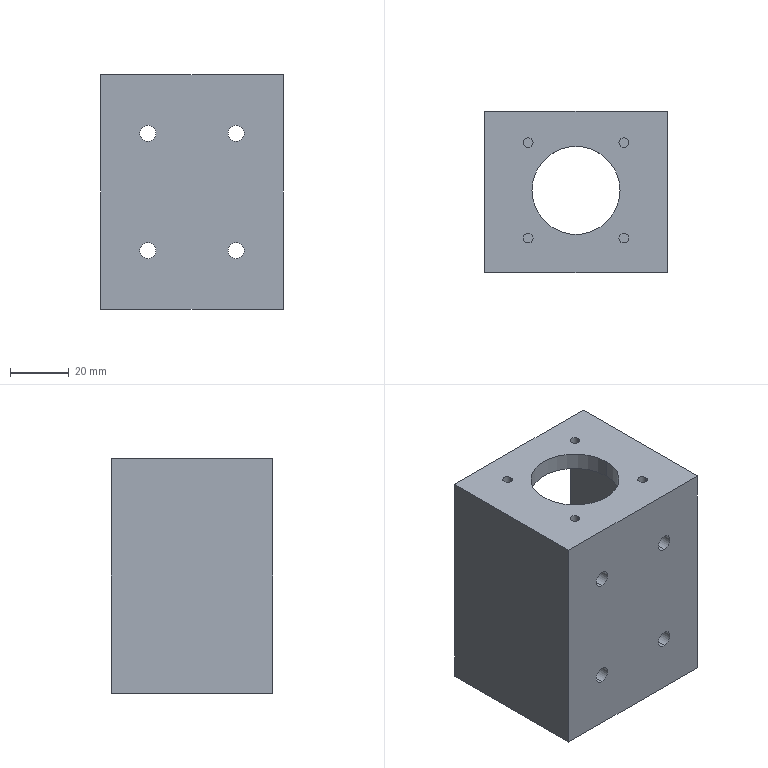Part | Creo | features CURVE 6, CUT 4, DATUM PLANE 3, PROTRUSION 2, CHAMFER 1, COORDINATE SYSTEM 1 | 1 solid | 45 faces | box 62 x 55 x 80 mm | volume 96326 mm3 | cylinder 26 | plane 19 | commonest cylinder face diameters 3.3 x8 5.5 x8 4.2 x6 30 x2 34 x2
STEP:
#1=CARTESIAN_POINT('',(0.,0.,0.));
#2=DIRECTION('',(0.,0.,1.));
#3=DIRECTION('',(1.,0.,0.));
#4=AXIS2_PLACEMENT_3D('',#1,#2,#3);
#5=CARTESIAN_POINT('',(31.,27.,0.));
#6=VERTEX_POINT('',#5);
#7=CARTESIAN_POINT('',(-31.,27.,0.));
#8=VERTEX_POINT('',#7);
#9=CARTESIAN_POINT('',(31.,27.,0.));
#10=DIRECTION('',(-1.,0.,0.));
#11=VECTOR('',#10,62.);
#12=LINE('',#9,#11);
#13=EDGE_CURVE('',#6,#8,#12,.T.);
#14=ORIENTED_EDGE('',*,*,#13,.T.);
#15=CARTESIAN_POINT('',(-31.,-28.,0.));
#16=VERTEX_POINT('',#15);
#17=CARTESIAN_POINT('',(-31.,27.,0.));
#18=DIRECTION('',(0.,-1.,0.));
#19=VECTOR('',#18,55.);
#20=LINE('',#17,#19);
#21=EDGE_CURVE('',#8,#16,#20,.T.);
#22=ORIENTED_EDGE('',*,*,#21,.T.);
#23=CARTESIAN_POINT('',(31.,-28.,0.));
#24=VERTEX_POINT('',#23);
#25=CARTESIAN_POINT('',(-31.,-28.,0.));
#26=DIRECTION('',(1.,0.,0.));
#27=VECTOR('',#26,62.);
#28=LINE('',#25,#27);
#29=EDGE_CURVE('',#16,#24,#28,.T.);
#30=ORIENTED_EDGE('',*,*,#29,.T.);
#31=CARTESIAN_POINT('',(31.,-28.,0.));
#32=DIRECTION('',(0.,1.,0.));
#33=VECTOR('',#32,55.);
#34=LINE('',#31,#33);
#35=EDGE_CURVE('',#24,#6,#34,.T.);
#36=ORIENTED_EDGE('',*,*,#35,.T.);
#37=EDGE_LOOP('',(#14,#22,#30,#36));
#38=FACE_OUTER_BOUND('',#37,.F.);
#39=CARTESIAN_POINT('',(0.,-17.,0.));
#40=VERTEX_POINT('',#39);
#41=CARTESIAN_POINT('',(0.,17.,0.));
#42=VERTEX_POINT('',#41);
#43=CARTESIAN_POINT('',(0.,0.,0.));
#44=DIRECTION('',(0.,0.,-1.));
#45=DIRECTION('',(0.,-1.,0.));
#46=AXIS2_PLACEMENT_3D('',#43,#44,#45);
#47=CIRCLE('',#46,17.);
#48=EDGE_CURVE('',#40,#42,#47,.T.);
#49=ORIENTED_EDGE('',*,*,#48,.T.);
#50=CARTESIAN_POINT('',(0.,0.,0.));
#51=DIRECTION('',(0.,0.,-1.));
#52=DIRECTION('',(0.,1.,0.));
#53=AXIS2_PLACEMENT_3D('',#50,#51,#52);
#54=CIRCLE('',#53,17.);
#55=EDGE_CURVE('',#42,#40,#54,.T.);
#56=ORIENTED_EDGE('',*,*,#55,.T.);
#57=EDGE_LOOP('',(#49,#56));
#58=FACE_BOUND('',#57,.F.);
#59=CARTESIAN_POINT('',(0.,18.9,0.));
#60=VERTEX_POINT('',#59);
#61=CARTESIAN_POINT('',(0.,23.1,0.));
#62=VERTEX_POINT('',#61);
#63=CARTESIAN_POINT('',(0.,21.,0.));
#64=DIRECTION('',(0.,0.,-1.));
#65=DIRECTION('',(0.,-1.,0.));
#66=AXIS2_PLACEMENT_3D('',#63,#64,#65);
#67=CIRCLE('',#66,2.1);
#68=EDGE_CURVE('',#60,#62,#67,.T.);
#69=ORIENTED_EDGE('',*,*,#68,.T.);
#70=CARTESIAN_POINT('',(0.,21.,0.));
#71=DIRECTION('',(0.,0.,-1.));
#72=DIRECTION('',(0.,1.,0.));
#73=AXIS2_PLACEMENT_3D('',#70,#71,#72);
#74=CIRCLE('',#73,2.1);
#75=EDGE_CURVE('',#62,#60,#74,.T.);
#76=ORIENTED_EDGE('',*,*,#75,.T.);
#77=EDGE_LOOP('',(#69,#76));
#78=FACE_BOUND('',#77,.F.);
#79=CARTESIAN_POINT('',(-18.187,-12.6,0.));
#80=VERTEX_POINT('',#79);
#81=CARTESIAN_POINT('',(-18.187,-8.4,0.));
#82=VERTEX_POINT('',#81);
#83=CARTESIAN_POINT('',(-18.187,-10.5,0.));
#84=DIRECTION('',(0.,0.,-1.));
#85=DIRECTION('',(0.,-1.,0.));
#86=AXIS2_PLACEMENT_3D('',#83,#84,#85);
#87=CIRCLE('',#86,2.1);
#88=EDGE_CURVE('',#80,#82,#87,.T.);
#89=ORIENTED_EDGE('',*,*,#88,.T.);
#90=CARTESIAN_POINT('',(-18.187,-10.5,0.));
#91=DIRECTION('',(0.,0.,-1.));
#92=DIRECTION('',(0.,1.,0.));
#93=AXIS2_PLACEMENT_3D('',#90,#91,#92);
#94=CIRCLE('',#93,2.1);
#95=EDGE_CURVE('',#82,#80,#94,.T.);
#96=ORIENTED_EDGE('',*,*,#95,.T.);
#97=EDGE_LOOP('',(#89,#96));
#98=FACE_BOUND('',#97,.F.);
#99=CARTESIAN_POINT('',(18.187,-12.6,0.));
#100=VERTEX_POINT('',#99);
#101=CARTESIAN_POINT('',(18.187,-8.4,0.));
#102=VERTEX_POINT('',#101);
#103=CARTESIAN_POINT('',(18.187,-10.5,0.));
#104=DIRECTION('',(0.,0.,-1.));
#105=DIRECTION('',(0.,-1.,0.));
#106=AXIS2_PLACEMENT_3D('',#103,#104,#105);
#107=CIRCLE('',#106,2.1);
#108=EDGE_CURVE('',#100,#102,#107,.T.);
#109=ORIENTED_EDGE('',*,*,#108,.T.);
#110=CARTESIAN_POINT('',(18.187,-10.5,0.));
#111=DIRECTION('',(0.,0.,-1.));
#112=DIRECTION('',(0.,1.,0.));
#113=AXIS2_PLACEMENT_3D('',#110,#111,#112);
#114=CIRCLE('',#113,2.1);
#115=EDGE_CURVE('',#102,#100,#114,.T.);
#116=ORIENTED_EDGE('',*,*,#115,.T.);
#117=EDGE_LOOP('',(#109,#116));
#118=FACE_BOUND('',#117,.F.);
#119=CARTESIAN_POINT('',(0.,0.,0.));
#120=DIRECTION('',(0.,0.,1.));
#121=DIRECTION('',(1.,0.,0.));
#122=AXIS2_PLACEMENT_3D('',#119,#120,#121);
#123=PLANE('',#122);
#124=ADVANCED_FACE('',(#38,#58,#78,#98,#118),#123,.F.);
#125=ORIENTED_EDGE('',*,*,#13,.F.);
#126=CARTESIAN_POINT('',(31.,27.,80.));
#127=VERTEX_POINT('',#126);
#128=CARTESIAN_POINT('',(31.,27.,0.));
#129=DIRECTION('',(0.,0.,1.));
#130=VECTOR('',#129,80.);
#131=LINE('',#128,#130);
#132=EDGE_CURVE('',#6,#127,#131,.T.);
#133=ORIENTED_EDGE('',*,*,#132,.T.);
#134=CARTESIAN_POINT('',(-31.,27.,80.));
#135=VERTEX_POINT('',#134);
#136=CARTESIAN_POINT('',(31.,27.,80.));
#137=DIRECTION('',(-1.,0.,0.));
#138=VECTOR('',#137,62.);
#139=LINE('',#136,#138);
#140=EDGE_CURVE('',#127,#135,#139,.T.);
#141=ORIENTED_EDGE('',*,*,#140,.T.);
#142=CARTESIAN_POINT('',(-31.,27.,0.));
#143=DIRECTION('',(0.,0.,1.));
#144=VECTOR('',#143,80.);
#145=LINE('',#142,#144);
#146=EDGE_CURVE('',#8,#135,#145,.T.);
#147=ORIENTED_EDGE('',*,*,#146,.F.);
#148=EDGE_LOOP('',(#125,#133,#141,#147));
#149=FACE_OUTER_BOUND('',#148,.F.);
#150=CARTESIAN_POINT('',(-25.,27.,8.));
#151=VERTEX_POINT('',#150);
#152=CARTESIAN_POINT('',(-25.,27.,72.));
#153=VERTEX_POINT('',#152);
#154=CARTESIAN_POINT('',(-25.,27.,8.));
#155=DIRECTION('',(0.,0.,1.));
#156=VECTOR('',#155,64.);
#157=LINE('',#154,#156);
#158=EDGE_CURVE('',#151,#153,#157,.T.);
#159=ORIENTED_EDGE('',*,*,#158,.T.);
#160=CARTESIAN_POINT('',(-23.,27.,74.));
#161=VERTEX_POINT('',#160);
#162=CARTESIAN_POINT('',(-23.,27.,74.));
#163=DIRECTION('',(-0.7071,0.,-0.7071));
#164=VECTOR('',#163,2.828);
#165=LINE('',#162,#164);
#166=EDGE_CURVE('',#161,#153,#165,.T.);
#167=ORIENTED_EDGE('',*,*,#166,.F.);
#168=CARTESIAN_POINT('',(23.,27.,74.));
#169=VERTEX_POINT('',#168);
#170=CARTESIAN_POINT('',(-23.,27.,74.));
#171=DIRECTION('',(1.,0.,0.));
#172=VECTOR('',#171,46.);
#173=LINE('',#170,#172);
#174=EDGE_CURVE('',#161,#169,#173,.T.);
#175=ORIENTED_EDGE('',*,*,#174,.T.);
#176=CARTESIAN_POINT('',(25.,27.,72.));
#177=VERTEX_POINT('',#176);
#178=CARTESIAN_POINT('',(25.,27.,72.));
#179=DIRECTION('',(-0.7071,0.,0.7071));
#180=VECTOR('',#179,2.828);
#181=LINE('',#178,#180);
#182=EDGE_CURVE('',#177,#169,#181,.T.);
#183=ORIENTED_EDGE('',*,*,#182,.F.);
#184=CARTESIAN_POINT('',(25.,27.,8.));
#185=VERTEX_POINT('',#184);
#186=CARTESIAN_POINT('',(25.,27.,72.));
#187=DIRECTION('',(0.,0.,-1.));
#188=VECTOR('',#187,64.);
#189=LINE('',#186,#188);
#190=EDGE_CURVE('',#177,#185,#189,.T.);
#191=ORIENTED_EDGE('',*,*,#190,.T.);
#192=CARTESIAN_POINT('',(23.,27.,6.));
#193=VERTEX_POINT('',#192);
#194=CARTESIAN_POINT('',(23.,27.,6.));
#195=DIRECTION('',(0.7071,0.,0.7071));
#196=VECTOR('',#195,2.828);
#197=LINE('',#194,#196);
#198=EDGE_CURVE('',#193,#185,#197,.T.);
#199=ORIENTED_EDGE('',*,*,#198,.F.);
#200=CARTESIAN_POINT('',(-23.,27.,6.));
#201=VERTEX_POINT('',#200);
#202=CARTESIAN_POINT('',(23.,27.,6.));
#203=DIRECTION('',(-1.,0.,0.));
#204=VECTOR('',#203,46.);
#205=LINE('',#202,#204);
#206=EDGE_CURVE('',#193,#201,#205,.T.);
#207=ORIENTED_EDGE('',*,*,#206,.T.);
#208=CARTESIAN_POINT('',(-25.,27.,8.));
#209=DIRECTION('',(0.7071,0.,-0.7071));
#210=VECTOR('',#209,2.828);
#211=LINE('',#208,#210);
#212=EDGE_CURVE('',#151,#201,#211,.T.);
#213=ORIENTED_EDGE('',*,*,#212,.F.);
#214=EDGE_LOOP('',(#159,#167,#175,#183,#191,#199,#207,#213));
#215=FACE_BOUND('',#214,.F.);
#216=CARTESIAN_POINT('',(31.,27.,0.));
#217=DIRECTION('',(0.,1.,0.));
#218=DIRECTION('',(-1.,0.,0.));
#219=AXIS2_PLACEMENT_3D('',#216,#217,#218);
#220=PLANE('',#219);
#221=ADVANCED_FACE('',(#149,#215),#220,.T.);
#222=ORIENTED_EDGE('',*,*,#35,.F.);
#223=CARTESIAN_POINT('',(31.,-28.,80.));
#224=VERTEX_POINT('',#223);
#225=CARTESIAN_POINT('',(31.,-28.,0.));
#226=DIRECTION('',(0.,0.,1.));
#227=VECTOR('',#226,80.);
#228=LINE('',#225,#227);
#229=EDGE_CURVE('',#24,#224,#228,.T.);
#230=ORIENTED_EDGE('',*,*,#229,.T.);
#231=CARTESIAN_POINT('',(31.,-28.,80.));
#232=DIRECTION('',(0.,1.,0.));
#233=VECTOR('',#232,55.);
#234=LINE('',#231,#233);
#235=EDGE_CURVE('',#224,#127,#234,.T.);
#236=ORIENTED_EDGE('',*,*,#235,.T.);
#237=ORIENTED_EDGE('',*,*,#132,.F.);
#238=EDGE_LOOP('',(#222,#230,#236,#237));
#239=FACE_OUTER_BOUND('',#238,.F.);
#240=CARTESIAN_POINT('',(31.,-28.,0.));
#241=DIRECTION('',(1.,0.,0.));
#242=DIRECTION('',(0.,1.,0.));
#243=AXIS2_PLACEMENT_3D('',#240,#241,#242);
#244=PLANE('',#243);
#245=ADVANCED_FACE('',(#239),#244,.T.);
#246=ORIENTED_EDGE('',*,*,#29,.F.);
#247=CARTESIAN_POINT('',(-31.,-28.,80.));
#248=VERTEX_POINT('',#247);
#249=CARTESIAN_POINT('',(-31.,-28.,0.));
#250=DIRECTION('',(0.,0.,1.));
#251=VECTOR('',#250,80.);
#252=LINE('',#249,#251);
#253=EDGE_CURVE('',#16,#248,#252,.T.);
#254=ORIENTED_EDGE('',*,*,#253,.T.);
#255=CARTESIAN_POINT('',(-31.,-28.,80.));
#256=DIRECTION('',(1.,0.,0.));
#257=VECTOR('',#256,62.);
#258=LINE('',#255,#257);
#259=EDGE_CURVE('',#248,#224,#258,.T.);
#260=ORIENTED_EDGE('',*,*,#259,.T.);
#261=ORIENTED_EDGE('',*,*,#229,.F.);
#262=EDGE_LOOP('',(#246,#254,#260,#261));
#263=FACE_OUTER_BOUND('',#262,.F.);
#264=CARTESIAN_POINT('',(-15.,-28.,57.25));
#265=VERTEX_POINT('',#264);
#266=CARTESIAN_POINT('',(-15.,-28.,62.75));
#267=VERTEX_POINT('',#266);
#268=CARTESIAN_POINT('',(-15.,-28.,60.));
#269=DIRECTION('',(0.,1.,0.));
#270=DIRECTION('',(0.,0.,-1.));
#271=AXIS2_PLACEMENT_3D('',#268,#269,#270);
#272=CIRCLE('',#271,2.75);
#273=EDGE_CURVE('',#265,#267,#272,.T.);
#274=ORIENTED_EDGE('',*,*,#273,.F.);
#275=CARTESIAN_POINT('',(-15.,-28.,60.));
#276=DIRECTION('',(0.,1.,0.));
#277=DIRECTION('',(0.,0.,1.));
#278=AXIS2_PLACEMENT_3D('',#275,#276,#277);
#279=CIRCLE('',#278,2.75);
#280=EDGE_CURVE('',#267,#265,#279,.T.);
#281=ORIENTED_EDGE('',*,*,#280,.F.);
#282=EDGE_LOOP('',(#274,#281));
#283=FACE_BOUND('',#282,.F.);
#284=CARTESIAN_POINT('',(-15.,-28.,17.25));
#285=VERTEX_POINT('',#284);
#286=CARTESIAN_POINT('',(-15.,-28.,22.75));
#287=VERTEX_POINT('',#286);
#288=CARTESIAN_POINT('',(-15.,-28.,20.));
#289=DIRECTION('',(0.,1.,0.));
#290=DIRECTION('',(0.,0.,-1.));
#291=AXIS2_PLACEMENT_3D('',#288,#289,#290);
#292=CIRCLE('',#291,2.75);
#293=EDGE_CURVE('',#285,#287,#292,.T.);
#294=ORIENTED_EDGE('',*,*,#293,.F.);
#295=CARTESIAN_POINT('',(-15.,-28.,20.));
#296=DIRECTION('',(0.,1.,0.));
#297=DIRECTION('',(0.,0.,1.));
#298=AXIS2_PLACEMENT_3D('',#295,#296,#297);
#299=CIRCLE('',#298,2.75);
#300=EDGE_CURVE('',#287,#285,#299,.T.);
#301=ORIENTED_EDGE('',*,*,#300,.F.);
#302=EDGE_LOOP('',(#294,#301));
#303=FACE_BOUND('',#302,.F.);
#304=CARTESIAN_POINT('',(15.,-28.,17.25));
#305=VERTEX_POINT('',#304);
#306=CARTESIAN_POINT('',(15.,-28.,22.75));
#307=VERTEX_POINT('',#306);
#308=CARTESIAN_POINT('',(15.,-28.,20.));
#309=DIRECTION('',(0.,1.,0.));
#310=DIRECTION('',(0.,0.,-1.));
#311=AXIS2_PLACEMENT_3D('',#308,#309,#310);
#312=CIRCLE('',#311,2.75);
#313=EDGE_CURVE('',#305,#307,#312,.T.);
#314=ORIENTED_EDGE('',*,*,#313,.F.);
#315=CARTESIAN_POINT('',(15.,-28.,20.));
#316=DIRECTION('',(0.,1.,0.));
#317=DIRECTION('',(0.,0.,1.));
#318=AXIS2_PLACEMENT_3D('',#315,#316,#317);
#319=CIRCLE('',#318,2.75);
#320=EDGE_CURVE('',#307,#305,#319,.T.);
#321=ORIENTED_EDGE('',*,*,#320,.F.);
#322=EDGE_LOOP('',(#314,#321));
#323=FACE_BOUND('',#322,.F.);
#324=CARTESIAN_POINT('',(15.,-28.,57.25));
#325=VERTEX_POINT('',#324);
#326=CARTESIAN_POINT('',(15.,-28.,62.75));
#327=VERTEX_POINT('',#326);
#328=CARTESIAN_POINT('',(15.,-28.,60.));
#329=DIRECTION('',(0.,1.,0.));
#330=DIRECTION('',(0.,0.,-1.));
#331=AXIS2_PLACEMENT_3D('',#328,#329,#330);
#332=CIRCLE('',#331,2.75);
#333=EDGE_CURVE('',#325,#327,#332,.T.);
#334=ORIENTED_EDGE('',*,*,#333,.F.);
#335=CARTESIAN_POINT('',(15.,-28.,60.));
#336=DIRECTION('',(0.,1.,0.));
#337=DIRECTION('',(0.,0.,1.));
#338=AXIS2_PLACEMENT_3D('',#335,#336,#337);
#339=CIRCLE('',#338,2.75);
#340=EDGE_CURVE('',#327,#325,#339,.T.);
#341=ORIENTED_EDGE('',*,*,#340,.F.);
#342=EDGE_LOOP('',(#334,#341));
#343=FACE_BOUND('',#342,.F.);
#344=CARTESIAN_POINT('',(-31.,-28.,0.));
#345=DIRECTION('',(0.,-1.,0.));
#346=DIRECTION('',(1.,0.,0.));
#347=AXIS2_PLACEMENT_3D('',#344,#345,#346);
#348=PLANE('',#347);
#349=ADVANCED_FACE('',(#263,#283,#303,#323,#343),#348,.T.);
#350=ORIENTED_EDGE('',*,*,#21,.F.);
#351=ORIENTED_EDGE('',*,*,#146,.T.);
#352=CARTESIAN_POINT('',(-31.,27.,80.));
#353=DIRECTION('',(0.,-1.,0.));
#354=VECTOR('',#353,55.);
#355=LINE('',#352,#354);
#356=EDGE_CURVE('',#135,#248,#355,.T.);
#357=ORIENTED_EDGE('',*,*,#356,.T.);
#358=ORIENTED_EDGE('',*,*,#253,.F.);
#359=EDGE_LOOP('',(#350,#351,#357,#358));
#360=FACE_OUTER_BOUND('',#359,.F.);
#361=CARTESIAN_POINT('',(-31.,27.,0.));
#362=DIRECTION('',(-1.,0.,0.));
#363=DIRECTION('',(0.,-1.,0.));
#364=AXIS2_PLACEMENT_3D('',#361,#362,#363);
#365=PLANE('',#364);
#366=ADVANCED_FACE('',(#360),#365,.T.);
#367=ORIENTED_EDGE('',*,*,#140,.F.);
#368=ORIENTED_EDGE('',*,*,#235,.F.);
#369=ORIENTED_EDGE('',*,*,#259,.F.);
#370=ORIENTED_EDGE('',*,*,#356,.F.);
#371=EDGE_LOOP('',(#367,#368,#369,#370));
#372=FACE_OUTER_BOUND('',#371,.F.);
#373=CARTESIAN_POINT('',(-14.61,16.26,80.));
#374=VERTEX_POINT('',#373);
#375=CARTESIAN_POINT('',(-17.91,16.26,80.));
#376=VERTEX_POINT('',#375);
#377=CARTESIAN_POINT('',(-16.26,16.26,80.));
#378=DIRECTION('',(0.,0.,-1.));
#379=DIRECTION('',(1.,0.,0.));
#380=AXIS2_PLACEMENT_3D('',#377,#378,#379);
#381=CIRCLE('',#380,1.65);
#382=EDGE_CURVE('',#374,#376,#381,.T.);
#383=ORIENTED_EDGE('',*,*,#382,.F.);
#384=CARTESIAN_POINT('',(-16.26,16.26,80.));
#385=DIRECTION('',(0.,0.,-1.));
#386=DIRECTION('',(-1.,0.,0.));
#387=AXIS2_PLACEMENT_3D('',#384,#385,#386);
#388=CIRCLE('',#387,1.65);
#389=EDGE_CURVE('',#376,#374,#388,.T.);
#390=ORIENTED_EDGE('',*,*,#389,.F.);
#391=EDGE_LOOP('',(#383,#390));
#392=FACE_BOUND('',#391,.F.);
#393=CARTESIAN_POINT('',(17.91,16.26,80.));
#394=VERTEX_POINT('',#393);
#395=CARTESIAN_POINT('',(14.61,16.26,80.));
#396=VERTEX_POINT('',#395);
#397=CARTESIAN_POINT('',(16.26,16.26,80.));
#398=DIRECTION('',(0.,0.,-1.));
#399=DIRECTION('',(1.,0.,0.));
#400=AXIS2_PLACEMENT_3D('',#397,#398,#399);
#401=CIRCLE('',#400,1.65);
#402=EDGE_CURVE('',#394,#396,#401,.T.);
#403=ORIENTED_EDGE('',*,*,#402,.F.);
#404=CARTESIAN_POINT('',(16.26,16.26,80.));
#405=DIRECTION('',(0.,0.,-1.));
#406=DIRECTION('',(-1.,0.,0.));
#407=AXIS2_PLACEMENT_3D('',#404,#405,#406);
#408=CIRCLE('',#407,1.65);
#409=EDGE_CURVE('',#396,#394,#408,.T.);
#410=ORIENTED_EDGE('',*,*,#409,.F.);
#411=EDGE_LOOP('',(#403,#410));
#412=FACE_BOUND('',#411,.F.);
#413=CARTESIAN_POINT('',(17.91,-16.26,80.));
#414=VERTEX_POINT('',#413);
#415=CARTESIAN_POINT('',(14.61,-16.26,80.));
#416=VERTEX_POINT('',#415);
#417=CARTESIAN_POINT('',(16.26,-16.26,80.));
#418=DIRECTION('',(0.,0.,-1.));
#419=DIRECTION('',(1.,0.,0.));
#420=AXIS2_PLACEMENT_3D('',#417,#418,#419);
#421=CIRCLE('',#420,1.65);
#422=EDGE_CURVE('',#414,#416,#421,.T.);
#423=ORIENTED_EDGE('',*,*,#422,.F.);
#424=CARTESIAN_POINT('',(16.26,-16.26,80.));
#425=DIRECTION('',(0.,0.,-1.));
#426=DIRECTION('',(-1.,0.,0.));
#427=AXIS2_PLACEMENT_3D('',#424,#425,#426);
#428=CIRCLE('',#427,1.65);
#429=EDGE_CURVE('',#416,#414,#428,.T.);
#430=ORIENTED_EDGE('',*,*,#429,.F.);
#431=EDGE_LOOP('',(#423,#430));
#432=FACE_BOUND('',#431,.F.);
#433=CARTESIAN_POINT('',(-14.61,-16.26,80.));
#434=VERTEX_POINT('',#433);
#435=CARTESIAN_POINT('',(-17.91,-16.26,80.));
#436=VERTEX_POINT('',#435);
#437=CARTESIAN_POINT('',(-16.26,-16.26,80.));
#438=DIRECTION('',(0.,0.,-1.));
#439=DIRECTION('',(1.,0.,0.));
#440=AXIS2_PLACEMENT_3D('',#437,#438,#439);
#441=CIRCLE('',#440,1.65);
#442=EDGE_CURVE('',#434,#436,#441,.T.);
#443=ORIENTED_EDGE('',*,*,#442,.F.);
#444=CARTESIAN_POINT('',(-16.26,-16.26,80.));
#445=DIRECTION('',(0.,0.,-1.));
#446=DIRECTION('',(-1.,0.,0.));
#447=AXIS2_PLACEMENT_3D('',#444,#445,#446);
#448=CIRCLE('',#447,1.65);
#449=EDGE_CURVE('',#436,#434,#448,.T.);
#450=ORIENTED_EDGE('',*,*,#449,.F.);
#451=EDGE_LOOP('',(#443,#450));
#452=FACE_BOUND('',#451,.F.);
#453=CARTESIAN_POINT('',(15.,0.,80.));
#454=VERTEX_POINT('',#453);
#455=CARTESIAN_POINT('',(-15.,0.,80.));
#456=VERTEX_POINT('',#455);
#457=CARTESIAN_POINT('',(0.,0.,80.));
#458=DIRECTION('',(0.,0.,-1.));
#459=DIRECTION('',(1.,0.,0.));
#460=AXIS2_PLACEMENT_3D('',#457,#458,#459);
#461=CIRCLE('',#460,15.);
#462=EDGE_CURVE('',#454,#456,#461,.T.);
#463=ORIENTED_EDGE('',*,*,#462,.F.);
#464=CARTESIAN_POINT('',(0.,0.,80.));
#465=DIRECTION('',(0.,0.,-1.));
#466=DIRECTION('',(-1.,0.,0.));
#467=AXIS2_PLACEMENT_3D('',#464,#465,#466);
#468=CIRCLE('',#467,15.);
#469=EDGE_CURVE('',#456,#454,#468,.T.);
#470=ORIENTED_EDGE('',*,*,#469,.F.);
#471=EDGE_LOOP('',(#463,#470));
#472=FACE_BOUND('',#471,.F.);
#473=CARTESIAN_POINT('',(0.,0.,80.));
#474=DIRECTION('',(0.,0.,1.));
#475=DIRECTION('',(1.,0.,0.));
#476=AXIS2_PLACEMENT_3D('',#473,#474,#475);
#477=PLANE('',#476);
#478=ADVANCED_FACE('',(#372,#392,#412,#432,#452,#472),#477,.T.);
#479=CARTESIAN_POINT('',(-15.,0.,74.));
#480=VERTEX_POINT('',#479);
#481=CARTESIAN_POINT('',(15.,0.,74.));
#482=VERTEX_POINT('',#481);
#483=CARTESIAN_POINT('',(0.,0.,74.));
#484=DIRECTION('',(0.,0.,1.));
#485=DIRECTION('',(-1.,0.,0.));
#486=AXIS2_PLACEMENT_3D('',#483,#484,#485);
#487=CIRCLE('',#486,15.);
#488=EDGE_CURVE('',#480,#482,#487,.T.);
#489=ORIENTED_EDGE('',*,*,#488,.T.);
#490=CARTESIAN_POINT('',(15.,0.,74.));
#491=DIRECTION('',(0.,0.,1.));
#492=VECTOR('',#491,6.);
#493=LINE('',#490,#492);
#494=EDGE_CURVE('',#482,#454,#493,.T.);
#495=ORIENTED_EDGE('',*,*,#494,.T.);
#496=ORIENTED_EDGE('',*,*,#462,.T.);
#497=CARTESIAN_POINT('',(-15.,0.,74.));
#498=DIRECTION('',(0.,0.,1.));
#499=VECTOR('',#498,6.);
#500=LINE('',#497,#499);
#501=EDGE_CURVE('',#480,#456,#500,.T.);
#502=ORIENTED_EDGE('',*,*,#501,.F.);
#503=EDGE_LOOP('',(#489,#495,#496,#502));
#504=FACE_OUTER_BOUND('',#503,.F.);
#505=CARTESIAN_POINT('',(0.,0.,0.));
#506=DIRECTION('',(0.,0.,1.));
#507=DIRECTION('',(1.,0.,0.));
#508=AXIS2_PLACEMENT_3D('',#505,#506,#507);
#509=CYLINDRICAL_SURFACE('',#508,15.);
#510=ADVANCED_FACE('',(#504),#509,.F.);
#511=CARTESIAN_POINT('',(23.,-20.,74.));
#512=VERTEX_POINT('',#511);
#513=CARTESIAN_POINT('',(23.,27.,74.));
#514=DIRECTION('',(0.,-1.,0.));
#515=VECTOR('',#514,47.);
#516=LINE('',#513,#515);
#517=EDGE_CURVE('',#169,#512,#516,.T.);
#518=ORIENTED_EDGE('',*,*,#517,.F.);
#519=ORIENTED_EDGE('',*,*,#174,.F.);
#520=CARTESIAN_POINT('',(-23.,-20.,74.));
#521=VERTEX_POINT('',#520);
#522=CARTESIAN_POINT('',(-23.,27.,74.));
#523=DIRECTION('',(0.,-1.,0.));
#524=VECTOR('',#523,47.);
#525=LINE('',#522,#524);
#526=EDGE_CURVE('',#161,#521,#525,.T.);
#527=ORIENTED_EDGE('',*,*,#526,.T.);
#528=CARTESIAN_POINT('',(23.,-20.,74.));
#529=DIRECTION('',(-1.,0.,0.));
#530=VECTOR('',#529,46.);
#531=LINE('',#528,#530);
#532=EDGE_CURVE('',#512,#521,#531,.T.);
#533=ORIENTED_EDGE('',*,*,#532,.F.);
#534=EDGE_LOOP('',(#518,#519,#527,#533));
#535=FACE_OUTER_BOUND('',#534,.F.);
#536=CARTESIAN_POINT('',(-17.91,16.26,74.));
#537=VERTEX_POINT('',#536);
#538=CARTESIAN_POINT('',(-14.61,16.26,74.));
#539=VERTEX_POINT('',#538);
#540=CARTESIAN_POINT('',(-16.26,16.26,74.));
#541=DIRECTION('',(0.,0.,1.));
#542=DIRECTION('',(-1.,0.,0.));
#543=AXIS2_PLACEMENT_3D('',#540,#541,#542);
#544=CIRCLE('',#543,1.65);
#545=EDGE_CURVE('',#537,#539,#544,.T.);
#546=ORIENTED_EDGE('',*,*,#545,.F.);
#547=CARTESIAN_POINT('',(-16.26,16.26,74.));
#548=DIRECTION('',(0.,0.,1.));
#549=DIRECTION('',(1.,0.,0.));
#550=AXIS2_PLACEMENT_3D('',#547,#548,#549);
#551=CIRCLE('',#550,1.65);
#552=EDGE_CURVE('',#539,#537,#551,.T.);
#553=ORIENTED_EDGE('',*,*,#552,.F.);
#554=EDGE_LOOP('',(#546,#553));
#555=FACE_BOUND('',#554,.F.);
#556=CARTESIAN_POINT('',(14.61,16.26,74.));
#557=VERTEX_POINT('',#556);
#558=CARTESIAN_POINT('',(17.91,16.26,74.));
#559=VERTEX_POINT('',#558);
#560=CARTESIAN_POINT('',(16.26,16.26,74.));
#561=DIRECTION('',(0.,0.,1.));
#562=DIRECTION('',(-1.,0.,0.));
#563=AXIS2_PLACEMENT_3D('',#560,#561,#562);
#564=CIRCLE('',#563,1.65);
#565=EDGE_CURVE('',#557,#559,#564,.T.);
#566=ORIENTED_EDGE('',*,*,#565,.F.);
#567=CARTESIAN_POINT('',(16.26,16.26,74.));
#568=DIRECTION('',(0.,0.,1.));
#569=DIRECTION('',(1.,0.,0.));
#570=AXIS2_PLACEMENT_3D('',#567,#568,#569);
#571=CIRCLE('',#570,1.65);
#572=EDGE_CURVE('',#559,#557,#571,.T.);
#573=ORIENTED_EDGE('',*,*,#572,.F.);
#574=EDGE_LOOP('',(#566,#573));
#575=FACE_BOUND('',#574,.F.);
#576=CARTESIAN_POINT('',(14.61,-16.26,74.));
#577=VERTEX_POINT('',#576);
#578=CARTESIAN_POINT('',(17.91,-16.26,74.));
#579=VERTEX_POINT('',#578);
#580=CARTESIAN_POINT('',(16.26,-16.26,74.));
#581=DIRECTION('',(0.,0.,1.));
#582=DIRECTION('',(-1.,0.,0.));
#583=AXIS2_PLACEMENT_3D('',#580,#581,#582);
#584=CIRCLE('',#583,1.65);
#585=EDGE_CURVE('',#577,#579,#584,.T.);
#586=ORIENTED_EDGE('',*,*,#585,.F.);
#587=CARTESIAN_POINT('',(16.26,-16.26,74.));
#588=DIRECTION('',(0.,0.,1.));
#589=DIRECTION('',(1.,0.,0.));
#590=AXIS2_PLACEMENT_3D('',#587,#588,#589);
#591=CIRCLE('',#590,1.65);
#592=EDGE_CURVE('',#579,#577,#591,.T.);
#593=ORIENTED_EDGE('',*,*,#592,.F.);
#594=EDGE_LOOP('',(#586,#593));
#595=FACE_BOUND('',#594,.F.);
#596=CARTESIAN_POINT('',(-17.91,-16.26,74.));
#597=VERTEX_POINT('',#596);
#598=CARTESIAN_POINT('',(-14.61,-16.26,74.));
#599=VERTEX_POINT('',#598);
#600=CARTESIAN_POINT('',(-16.26,-16.26,74.));
#601=DIRECTION('',(0.,0.,1.));
#602=DIRECTION('',(-1.,0.,0.));
#603=AXIS2_PLACEMENT_3D('',#600,#601,#602);
#604=CIRCLE('',#603,1.65);
#605=EDGE_CURVE('',#597,#599,#604,.T.);
#606=ORIENTED_EDGE('',*,*,#605,.F.);
#607=CARTESIAN_POINT('',(-16.26,-16.26,74.));
#608=DIRECTION('',(0.,0.,1.));
#609=DIRECTION('',(1.,0.,0.));
#610=AXIS2_PLACEMENT_3D('',#607,#608,#609);
#611=CIRCLE('',#610,1.65);
#612=EDGE_CURVE('',#599,#597,#611,.T.);
#613=ORIENTED_EDGE('',*,*,#612,.F.);
#614=EDGE_LOOP('',(#606,#613));
#615=FACE_BOUND('',#614,.F.);
#616=ORIENTED_EDGE('',*,*,#488,.F.);
#617=CARTESIAN_POINT('',(0.,0.,74.));
#618=DIRECTION('',(0.,0.,1.));
#619=DIRECTION('',(1.,0.,0.));
#620=AXIS2_PLACEMENT_3D('',#617,#618,#619);
#621=CIRCLE('',#620,15.);
#622=EDGE_CURVE('',#482,#480,#621,.T.);
#623=ORIENTED_EDGE('',*,*,#622,.F.);
#624=EDGE_LOOP('',(#616,#623));
#625=FACE_BOUND('',#624,.F.);
#626=CARTESIAN_POINT('',(-25.,27.,74.));
#627=DIRECTION('',(0.,0.,1.));
#628=DIRECTION('',(1.,0.,0.));
#629=AXIS2_PLACEMENT_3D('',#626,#627,#628);
#630=PLANE('',#629);
#631=ADVANCED_FACE('',(#535,#555,#575,#595,#615,#625),#630,.F.);
#632=ORIENTED_EDGE('',*,*,#622,.T.);
#633=ORIENTED_EDGE('',*,*,#501,.T.);
#634=ORIENTED_EDGE('',*,*,#469,.T.);
#635=ORIENTED_EDGE('',*,*,#494,.F.);
#636=EDGE_LOOP('',(#632,#633,#634,#635));
#637=FACE_OUTER_BOUND('',#636,.F.);
#638=CARTESIAN_POINT('',(0.,0.,0.));
#639=DIRECTION('',(0.,0.,1.));
#640=DIRECTION('',(1.,0.,0.));
#641=AXIS2_PLACEMENT_3D('',#638,#639,#640);
#642=CYLINDRICAL_SURFACE('',#641,15.);
#643=ADVANCED_FACE('',(#637),#642,.F.);
#644=ORIENTED_EDGE('',*,*,#545,.T.);
#645=CARTESIAN_POINT('',(-14.61,16.26,74.));
#646=DIRECTION('',(0.,0.,1.));
#647=VECTOR('',#646,6.);
#648=LINE('',#645,#647);
#649=EDGE_CURVE('',#539,#374,#648,.T.);
#650=ORIENTED_EDGE('',*,*,#649,.T.);
#651=ORIENTED_EDGE('',*,*,#382,.T.);
#652=CARTESIAN_POINT('',(-17.91,16.26,74.));
#653=DIRECTION('',(0.,0.,1.));
#654=VECTOR('',#653,6.);
#655=LINE('',#652,#654);
#656=EDGE_CURVE('',#537,#376,#655,.T.);
#657=ORIENTED_EDGE('',*,*,#656,.F.);
#658=EDGE_LOOP('',(#644,#650,#651,#657));
#659=FACE_OUTER_BOUND('',#658,.F.);
#660=CARTESIAN_POINT('',(-16.26,16.26,0.));
#661=DIRECTION('',(0.,0.,1.));
#662=DIRECTION('',(1.,0.,0.));
#663=AXIS2_PLACEMENT_3D('',#660,#661,#662);
#664=CYLINDRICAL_SURFACE('',#663,1.65);
#665=ADVANCED_FACE('',(#659),#664,.F.);
#666=ORIENTED_EDGE('',*,*,#552,.T.);
#667=ORIENTED_EDGE('',*,*,#656,.T.);
#668=ORIENTED_EDGE('',*,*,#389,.T.);
#669=ORIENTED_EDGE('',*,*,#649,.F.);
#670=EDGE_LOOP('',(#666,#667,#668,#669));
#671=FACE_OUTER_BOUND('',#670,.F.);
#672=CARTESIAN_POINT('',(-16.26,16.26,0.));
#673=DIRECTION('',(0.,0.,1.));
#674=DIRECTION('',(1.,0.,0.));
#675=AXIS2_PLACEMENT_3D('',#672,#673,#674);
#676=CYLINDRICAL_SURFACE('',#675,1.65);
#677=ADVANCED_FACE('',(#671),#676,.F.);
#678=ORIENTED_EDGE('',*,*,#565,.T.);
#679=CARTESIAN_POINT('',(17.91,16.26,74.));
#680=DIRECTION('',(0.,0.,1.));
#681=VECTOR('',#680,6.);
#682=LINE('',#679,#681);
#683=EDGE_CURVE('',#559,#394,#682,.T.);
#684=ORIENTED_EDGE('',*,*,#683,.T.);
#685=ORIENTED_EDGE('',*,*,#402,.T.);
#686=CARTESIAN_POINT('',(14.61,16.26,74.));
#687=DIRECTION('',(0.,0.,1.));
#688=VECTOR('',#687,6.);
#689=LINE('',#686,#688);
#690=EDGE_CURVE('',#557,#396,#689,.T.);
#691=ORIENTED_EDGE('',*,*,#690,.F.);
#692=EDGE_LOOP('',(#678,#684,#685,#691));
#693=FACE_OUTER_BOUND('',#692,.F.);
#694=CARTESIAN_POINT('',(16.26,16.26,0.));
#695=DIRECTION('',(0.,0.,1.));
#696=DIRECTION('',(1.,0.,0.));
#697=AXIS2_PLACEMENT_3D('',#694,#695,#696);
#698=CYLINDRICAL_SURFACE('',#697,1.65);
#699=ADVANCED_FACE('',(#693),#698,.F.);
#700=ORIENTED_EDGE('',*,*,#572,.T.);
#701=ORIENTED_EDGE('',*,*,#690,.T.);
#702=ORIENTED_EDGE('',*,*,#409,.T.);
#703=ORIENTED_EDGE('',*,*,#683,.F.);
#704=EDGE_LOOP('',(#700,#701,#702,#703));
#705=FACE_OUTER_BOUND('',#704,.F.);
#706=CARTESIAN_POINT('',(16.26,16.26,0.));
#707=DIRECTION('',(0.,0.,1.));
#708=DIRECTION('',(1.,0.,0.));
#709=AXIS2_PLACEMENT_3D('',#706,#707,#708);
#710=CYLINDRICAL_SURFACE('',#709,1.65);
#711=ADVANCED_FACE('',(#705),#710,.F.);
#712=ORIENTED_EDGE('',*,*,#585,.T.);
#713=CARTESIAN_POINT('',(17.91,-16.26,74.));
#714=DIRECTION('',(0.,0.,1.));
#715=VECTOR('',#714,6.);
#716=LINE('',#713,#715);
#717=EDGE_CURVE('',#579,#414,#716,.T.);
#718=ORIENTED_EDGE('',*,*,#717,.T.);
#719=ORIENTED_EDGE('',*,*,#422,.T.);
#720=CARTESIAN_POINT('',(14.61,-16.26,74.));
#721=DIRECTION('',(0.,0.,1.));
#722=VECTOR('',#721,6.);
#723=LINE('',#720,#722);
#724=EDGE_CURVE('',#577,#416,#723,.T.);
#725=ORIENTED_EDGE('',*,*,#724,.F.);
#726=EDGE_LOOP('',(#712,#718,#719,#725));
#727=FACE_OUTER_BOUND('',#726,.F.);
#728=CARTESIAN_POINT('',(16.26,-16.26,0.));
#729=DIRECTION('',(0.,0.,1.));
#730=DIRECTION('',(1.,0.,0.));
#731=AXIS2_PLACEMENT_3D('',#728,#729,#730);
#732=CYLINDRICAL_SURFACE('',#731,1.65);
#733=ADVANCED_FACE('',(#727),#732,.F.);
#734=ORIENTED_EDGE('',*,*,#592,.T.);
#735=ORIENTED_EDGE('',*,*,#724,.T.);
#736=ORIENTED_EDGE('',*,*,#429,.T.);
#737=ORIENTED_EDGE('',*,*,#717,.F.);
#738=EDGE_LOOP('',(#734,#735,#736,#737));
#739=FACE_OUTER_BOUND('',#738,.F.);
#740=CARTESIAN_POINT('',(16.26,-16.26,0.));
#741=DIRECTION('',(0.,0.,1.));
#742=DIRECTION('',(1.,0.,0.));
#743=AXIS2_PLACEMENT_3D('',#740,#741,#742);
#744=CYLINDRICAL_SURFACE('',#743,1.65);
#745=ADVANCED_FACE('',(#739),#744,.F.);
#746=ORIENTED_EDGE('',*,*,#605,.T.);
#747=CARTESIAN_POINT('',(-14.61,-16.26,74.));
#748=DIRECTION('',(0.,0.,1.));
#749=VECTOR('',#748,6.);
#750=LINE('',#747,#749);
#751=EDGE_CURVE('',#599,#434,#750,.T.);
#752=ORIENTED_EDGE('',*,*,#751,.T.);
#753=ORIENTED_EDGE('',*,*,#442,.T.);
#754=CARTESIAN_POINT('',(-17.91,-16.26,74.));
#755=DIRECTION('',(0.,0.,1.));
#756=VECTOR('',#755,6.);
#757=LINE('',#754,#756);
#758=EDGE_CURVE('',#597,#436,#757,.T.);
#759=ORIENTED_EDGE('',*,*,#758,.F.);
#760=EDGE_LOOP('',(#746,#752,#753,#759));
#761=FACE_OUTER_BOUND('',#760,.F.);
#762=CARTESIAN_POINT('',(-16.26,-16.26,0.));
#763=DIRECTION('',(0.,0.,1.));
#764=DIRECTION('',(1.,0.,0.));
#765=AXIS2_PLACEMENT_3D('',#762,#763,#764);
#766=CYLINDRICAL_SURFACE('',#765,1.65);
#767=ADVANCED_FACE('',(#761),#766,.F.);
#768=ORIENTED_EDGE('',*,*,#612,.T.);
#769=ORIENTED_EDGE('',*,*,#758,.T.);
#770=ORIENTED_EDGE('',*,*,#449,.T.);
#771=ORIENTED_EDGE('',*,*,#751,.F.);
#772=EDGE_LOOP('',(#768,#769,#770,#771));
#773=FACE_OUTER_BOUND('',#772,.F.);
#774=CARTESIAN_POINT('',(-16.26,-16.26,0.));
#775=DIRECTION('',(0.,0.,1.));
#776=DIRECTION('',(1.,0.,0.));
#777=AXIS2_PLACEMENT_3D('',#774,#775,#776);
#778=CYLINDRICAL_SURFACE('',#777,1.65);
#779=ADVANCED_FACE('',(#773),#778,.F.);
#780=ORIENTED_EDGE('',*,*,#517,.T.);
#781=CARTESIAN_POINT('',(24.,-21.,73.));
#782=VERTEX_POINT('',#781);
#783=CARTESIAN_POINT('',(24.,-21.,73.));
#784=DIRECTION('',(-0.5774,0.5774,0.5774));
#785=VECTOR('',#784,1.732);
#786=LINE('',#783,#785);
#787=EDGE_CURVE('',#782,#512,#786,.T.);
#788=ORIENTED_EDGE('',*,*,#787,.F.);
#789=CARTESIAN_POINT('',(25.,-20.,72.));
#790=VERTEX_POINT('',#789);
#791=CARTESIAN_POINT('',(25.,-20.,72.));
#792=DIRECTION('',(-0.5774,-0.5774,0.5774));
#793=VECTOR('',#792,1.732);
#794=LINE('',#791,#793);
#795=EDGE_CURVE('',#790,#782,#794,.T.);
#796=ORIENTED_EDGE('',*,*,#795,.F.);
#797=CARTESIAN_POINT('',(25.,27.,72.));
#798=DIRECTION('',(0.,-1.,0.));
#799=VECTOR('',#798,47.);
#800=LINE('',#797,#799);
#801=EDGE_CURVE('',#177,#790,#800,.T.);
#802=ORIENTED_EDGE('',*,*,#801,.F.);
#803=ORIENTED_EDGE('',*,*,#182,.T.);
#804=EDGE_LOOP('',(#780,#788,#796,#802,#803));
#805=FACE_OUTER_BOUND('',#804,.F.);
#806=CARTESIAN_POINT('',(24.,2.5,73.));
#807=DIRECTION('',(-0.7071,0.,-0.7071));
#808=DIRECTION('',(0.7071,0.,-0.7071));
#809=AXIS2_PLACEMENT_3D('',#806,#807,#808);
#810=PLANE('',#809);
#811=ADVANCED_FACE('',(#805),#810,.T.);
#812=ORIENTED_EDGE('',*,*,#532,.T.);
#813=CARTESIAN_POINT('',(-24.,-21.,73.));
#814=VERTEX_POINT('',#813);
#815=CARTESIAN_POINT('',(-23.,-20.,74.));
#816=DIRECTION('',(-0.5774,-0.5774,-0.5774));
#817=VECTOR('',#816,1.732);
#818=LINE('',#815,#817);
#819=EDGE_CURVE('',#521,#814,#818,.T.);
#820=ORIENTED_EDGE('',*,*,#819,.T.);
#821=CARTESIAN_POINT('',(-23.,-22.,72.));
#822=VERTEX_POINT('',#821);
#823=CARTESIAN_POINT('',(-23.,-22.,72.));
#824=DIRECTION('',(-0.5774,0.5774,0.5774));
#825=VECTOR('',#824,1.732);
#826=LINE('',#823,#825);
#827=EDGE_CURVE('',#822,#814,#826,.T.);
#828=ORIENTED_EDGE('',*,*,#827,.F.);
#829=CARTESIAN_POINT('',(23.,-22.,72.));
#830=VERTEX_POINT('',#829);
#831=CARTESIAN_POINT('',(23.,-22.,72.));
#832=DIRECTION('',(-1.,0.,0.));
#833=VECTOR('',#832,46.);
#834=LINE('',#831,#833);
#835=EDGE_CURVE('',#830,#822,#834,.T.);
#836=ORIENTED_EDGE('',*,*,#835,.F.);
#837=CARTESIAN_POINT('',(23.,-22.,72.));
#838=DIRECTION('',(0.5774,0.5774,0.5774));
#839=VECTOR('',#838,1.732);
#840=LINE('',#837,#839);
#841=EDGE_CURVE('',#830,#782,#840,.T.);
#842=ORIENTED_EDGE('',*,*,#841,.T.);
#843=ORIENTED_EDGE('',*,*,#787,.T.);
#844=EDGE_LOOP('',(#812,#820,#828,#836,#842,#843));
#845=FACE_OUTER_BOUND('',#844,.F.);
#846=CARTESIAN_POINT('',(0.,-21.,73.));
#847=DIRECTION('',(0.,0.7071,-0.7071));
#848=DIRECTION('',(0.,-0.7071,-0.7071));
#849=AXIS2_PLACEMENT_3D('',#846,#847,#848);
#850=PLANE('',#849);
#851=ADVANCED_FACE('',(#845),#850,.T.);
#852=CARTESIAN_POINT('',(-25.,-20.,72.));
#853=VERTEX_POINT('',#852);
#854=CARTESIAN_POINT('',(-25.,27.,72.));
#855=DIRECTION('',(0.,-1.,0.));
#856=VECTOR('',#855,47.);
#857=LINE('',#854,#856);
#858=EDGE_CURVE('',#153,#853,#857,.T.);
#859=ORIENTED_EDGE('',*,*,#858,.T.);
#860=CARTESIAN_POINT('',(-24.,-21.,73.));
#861=DIRECTION('',(-0.5774,0.5774,-0.5774));
#862=VECTOR('',#861,1.732);
#863=LINE('',#860,#862);
#864=EDGE_CURVE('',#814,#853,#863,.T.);
#865=ORIENTED_EDGE('',*,*,#864,.F.);
#866=ORIENTED_EDGE('',*,*,#819,.F.);
#867=ORIENTED_EDGE('',*,*,#526,.F.);
#868=ORIENTED_EDGE('',*,*,#166,.T.);
#869=EDGE_LOOP('',(#859,#865,#866,#867,#868));
#870=FACE_OUTER_BOUND('',#869,.F.);
#871=CARTESIAN_POINT('',(-24.,2.5,73.));
#872=DIRECTION('',(0.7071,0.,-0.7071));
#873=DIRECTION('',(0.7071,0.,0.7071));
#874=AXIS2_PLACEMENT_3D('',#871,#872,#873);
#875=PLANE('',#874);
#876=ADVANCED_FACE('',(#870),#875,.T.);
#877=ORIENTED_EDGE('',*,*,#858,.F.);
#878=ORIENTED_EDGE('',*,*,#158,.F.);
#879=CARTESIAN_POINT('',(-25.,-20.,8.));
#880=VERTEX_POINT('',#879);
#881=CARTESIAN_POINT('',(-25.,27.,8.));
#882=DIRECTION('',(0.,-1.,0.));
#883=VECTOR('',#882,47.);
#884=LINE('',#881,#883);
#885=EDGE_CURVE('',#151,#880,#884,.T.);
#886=ORIENTED_EDGE('',*,*,#885,.T.);
#887=CARTESIAN_POINT('',(-25.,-20.,72.));
#888=DIRECTION('',(0.,0.,-1.));
#889=VECTOR('',#888,64.);
#890=LINE('',#887,#889);
#891=EDGE_CURVE('',#853,#880,#890,.T.);
#892=ORIENTED_EDGE('',*,*,#891,.F.);
#893=EDGE_LOOP('',(#877,#878,#886,#892));
#894=FACE_OUTER_BOUND('',#893,.F.);
#895=CARTESIAN_POINT('',(-25.,27.,6.));
#896=DIRECTION('',(-1.,0.,0.));
#897=DIRECTION('',(0.,0.,1.));
#898=AXIS2_PLACEMENT_3D('',#895,#896,#897);
#899=PLANE('',#898);
#900=ADVANCED_FACE('',(#894),#899,.F.);
#901=CARTESIAN_POINT('',(-23.,-20.,6.));
#902=VERTEX_POINT('',#901);
#903=CARTESIAN_POINT('',(-23.,27.,6.));
#904=DIRECTION('',(0.,-1.,0.));
#905=VECTOR('',#904,47.);
#906=LINE('',#903,#905);
#907=EDGE_CURVE('',#201,#902,#906,.T.);
#908=ORIENTED_EDGE('',*,*,#907,.T.);
#909=CARTESIAN_POINT('',(-24.,-21.,7.));
#910=VERTEX_POINT('',#909);
#911=CARTESIAN_POINT('',(-23.,-20.,6.));
#912=DIRECTION('',(-0.5774,-0.5774,0.5774));
#913=VECTOR('',#912,1.732);
#914=LINE('',#911,#913);
#915=EDGE_CURVE('',#902,#910,#914,.T.);
#916=ORIENTED_EDGE('',*,*,#915,.T.);
#917=CARTESIAN_POINT('',(-25.,-20.,8.));
#918=DIRECTION('',(0.5774,-0.5774,-0.5774));
#919=VECTOR('',#918,1.732);
#920=LINE('',#917,#919);
#921=EDGE_CURVE('',#880,#910,#920,.T.);
#922=ORIENTED_EDGE('',*,*,#921,.F.);
#923=ORIENTED_EDGE('',*,*,#885,.F.);
#924=ORIENTED_EDGE('',*,*,#212,.T.);
#925=EDGE_LOOP('',(#908,#916,#922,#923,#924));
#926=FACE_OUTER_BOUND('',#925,.F.);
#927=CARTESIAN_POINT('',(-24.,2.5,7.));
#928=DIRECTION('',(0.7071,0.,0.7071));
#929=DIRECTION('',(-0.7071,0.,0.7071));
#930=AXIS2_PLACEMENT_3D('',#927,#928,#929);
#931=PLANE('',#930);
#932=ADVANCED_FACE('',(#926),#931,.T.);
#933=ORIENTED_EDGE('',*,*,#907,.F.);
#934=ORIENTED_EDGE('',*,*,#206,.F.);
#935=CARTESIAN_POINT('',(23.,-20.,6.));
#936=VERTEX_POINT('',#935);
#937=CARTESIAN_POINT('',(23.,27.,6.));
#938=DIRECTION('',(0.,-1.,0.));
#939=VECTOR('',#938,47.);
#940=LINE('',#937,#939);
#941=EDGE_CURVE('',#193,#936,#940,.T.);
#942=ORIENTED_EDGE('',*,*,#941,.T.);
#943=CARTESIAN_POINT('',(-23.,-20.,6.));
#944=DIRECTION('',(1.,0.,0.));
#945=VECTOR('',#944,46.);
#946=LINE('',#943,#945);
#947=EDGE_CURVE('',#902,#936,#946,.T.);
#948=ORIENTED_EDGE('',*,*,#947,.F.);
#949=EDGE_LOOP('',(#933,#934,#942,#948));
#950=FACE_OUTER_BOUND('',#949,.F.);
#951=CARTESIAN_POINT('',(0.,18.9,6.));
#952=VERTEX_POINT('',#951);
#953=CARTESIAN_POINT('',(0.,23.1,6.));
#954=VERTEX_POINT('',#953);
#955=CARTESIAN_POINT('',(0.,21.,6.));
#956=DIRECTION('',(0.,0.,-1.));
#957=DIRECTION('',(0.,-1.,0.));
#958=AXIS2_PLACEMENT_3D('',#955,#956,#957);
#959=CIRCLE('',#958,2.1);
#960=EDGE_CURVE('',#952,#954,#959,.T.);
#961=ORIENTED_EDGE('',*,*,#960,.F.);
#962=CARTESIAN_POINT('',(0.,21.,6.));
#963=DIRECTION('',(0.,0.,-1.));
#964=DIRECTION('',(0.,1.,0.));
#965=AXIS2_PLACEMENT_3D('',#962,#963,#964);
#966=CIRCLE('',#965,2.1);
#967=EDGE_CURVE('',#954,#952,#966,.T.);
#968=ORIENTED_EDGE('',*,*,#967,.F.);
#969=EDGE_LOOP('',(#961,#968));
#970=FACE_BOUND('',#969,.F.);
#971=CARTESIAN_POINT('',(-18.187,-12.6,6.));
#972=VERTEX_POINT('',#971);
#973=CARTESIAN_POINT('',(-18.187,-8.4,6.));
#974=VERTEX_POINT('',#973);
#975=CARTESIAN_POINT('',(-18.187,-10.5,6.));
#976=DIRECTION('',(0.,0.,-1.));
#977=DIRECTION('',(0.,-1.,0.));
#978=AXIS2_PLACEMENT_3D('',#975,#976,#977);
#979=CIRCLE('',#978,2.1);
#980=EDGE_CURVE('',#972,#974,#979,.T.);
#981=ORIENTED_EDGE('',*,*,#980,.F.);
#982=CARTESIAN_POINT('',(-18.187,-10.5,6.));
#983=DIRECTION('',(0.,0.,-1.));
#984=DIRECTION('',(0.,1.,0.));
#985=AXIS2_PLACEMENT_3D('',#982,#983,#984);
#986=CIRCLE('',#985,2.1);
#987=EDGE_CURVE('',#974,#972,#986,.T.);
#988=ORIENTED_EDGE('',*,*,#987,.F.);
#989=EDGE_LOOP('',(#981,#988));
#990=FACE_BOUND('',#989,.F.);
#991=CARTESIAN_POINT('',(18.187,-12.6,6.));
#992=VERTEX_POINT('',#991);
#993=CARTESIAN_POINT('',(18.187,-8.4,6.));
#994=VERTEX_POINT('',#993);
#995=CARTESIAN_POINT('',(18.187,-10.5,6.));
#996=DIRECTION('',(0.,0.,-1.));
#997=DIRECTION('',(0.,-1.,0.));
#998=AXIS2_PLACEMENT_3D('',#995,#996,#997);
#999=CIRCLE('',#998,2.1);
#1000=EDGE_CURVE('',#992,#994,#999,.T.);
#1001=ORIENTED_EDGE('',*,*,#1000,.F.);
#1002=CARTESIAN_POINT('',(18.187,-10.5,6.));
#1003=DIRECTION('',(0.,0.,-1.));
#1004=DIRECTION('',(0.,1.,0.));
#1005=AXIS2_PLACEMENT_3D('',#1002,#1003,#1004);
#1006=CIRCLE('',#1005,2.1);
#1007=EDGE_CURVE('',#994,#992,#1006,.T.);
#1008=ORIENTED_EDGE('',*,*,#1007,.F.);
#1009=EDGE_LOOP('',(#1001,#1008));
#1010=FACE_BOUND('',#1009,.F.);
#1011=CARTESIAN_POINT('',(0.,-17.,6.));
#1012=VERTEX_POINT('',#1011);
#1013=CARTESIAN_POINT('',(0.,17.,6.));
#1014=VERTEX_POINT('',#1013);
#1015=CARTESIAN_POINT('',(0.,0.,6.));
#1016=DIRECTION('',(0.,0.,-1.));
#1017=DIRECTION('',(0.,-1.,0.));
#1018=AXIS2_PLACEMENT_3D('',#1015,#1016,#1017);
#1019=CIRCLE('',#1018,17.);
#1020=EDGE_CURVE('',#1012,#1014,#1019,.T.);
#1021=ORIENTED_EDGE('',*,*,#1020,.F.);
#1022=CARTESIAN_POINT('',(0.,0.,6.));
#1023=DIRECTION('',(0.,0.,-1.));
#1024=DIRECTION('',(0.,1.,0.));
#1025=AXIS2_PLACEMENT_3D('',#1022,#1023,#1024);
#1026=CIRCLE('',#1025,17.);
#1027=EDGE_CURVE('',#1014,#1012,#1026,.T.);
#1028=ORIENTED_EDGE('',*,*,#1027,.F.);
#1029=EDGE_LOOP('',(#1021,#1028));
#1030=FACE_BOUND('',#1029,.F.);
#1031=CARTESIAN_POINT('',(25.,27.,6.));
#1032=DIRECTION('',(0.,0.,-1.));
#1033=DIRECTION('',(-1.,0.,0.));
#1034=AXIS2_PLACEMENT_3D('',#1031,#1032,#1033);
#1035=PLANE('',#1034);
#1036=ADVANCED_FACE('',(#950,#970,#990,#1010,#1030),#1035,.F.);
#1037=ORIENTED_EDGE('',*,*,#48,.F.);
#1038=CARTESIAN_POINT('',(0.,-17.,0.));
#1039=DIRECTION('',(0.,0.,1.));
#1040=VECTOR('',#1039,6.);
#1041=LINE('',#1038,#1040);
#1042=EDGE_CURVE('',#40,#1012,#1041,.T.);
#1043=ORIENTED_EDGE('',*,*,#1042,.T.);
#1044=ORIENTED_EDGE('',*,*,#1020,.T.);
#1045=CARTESIAN_POINT('',(0.,17.,0.));
#1046=DIRECTION('',(0.,0.,1.));
#1047=VECTOR('',#1046,6.);
#1048=LINE('',#1045,#1047);
#1049=EDGE_CURVE('',#42,#1014,#1048,.T.);
#1050=ORIENTED_EDGE('',*,*,#1049,.F.);
#1051=EDGE_LOOP('',(#1037,#1043,#1044,#1050));
#1052=FACE_OUTER_BOUND('',#1051,.F.);
#1053=CARTESIAN_POINT('',(0.,0.,0.));
#1054=DIRECTION('',(0.,0.,-1.));
#1055=DIRECTION('',(0.,-1.,0.));
#1056=AXIS2_PLACEMENT_3D('',#1053,#1054,#1055);
#1057=CYLINDRICAL_SURFACE('',#1056,17.);
#1058=ADVANCED_FACE('',(#1052),#1057,.F.);
#1059=ORIENTED_EDGE('',*,*,#55,.F.);
#1060=ORIENTED_EDGE('',*,*,#1049,.T.);
#1061=ORIENTED_EDGE('',*,*,#1027,.T.);
#1062=ORIENTED_EDGE('',*,*,#1042,.F.);
#1063=EDGE_LOOP('',(#1059,#1060,#1061,#1062));
#1064=FACE_OUTER_BOUND('',#1063,.F.);
#1065=CARTESIAN_POINT('',(0.,0.,0.));
#1066=DIRECTION('',(0.,0.,-1.));
#1067=DIRECTION('',(0.,-1.,0.));
#1068=AXIS2_PLACEMENT_3D('',#1065,#1066,#1067);
#1069=CYLINDRICAL_SURFACE('',#1068,17.);
#1070=ADVANCED_FACE('',(#1064),#1069,.F.);
#1071=ORIENTED_EDGE('',*,*,#68,.F.);
#1072=CARTESIAN_POINT('',(0.,18.9,0.));
#1073=DIRECTION('',(0.,0.,1.));
#1074=VECTOR('',#1073,6.);
#1075=LINE('',#1072,#1074);
#1076=EDGE_CURVE('',#60,#952,#1075,.T.);
#1077=ORIENTED_EDGE('',*,*,#1076,.T.);
#1078=ORIENTED_EDGE('',*,*,#960,.T.);
#1079=CARTESIAN_POINT('',(0.,23.1,0.));
#1080=DIRECTION('',(0.,0.,1.));
#1081=VECTOR('',#1080,6.);
#1082=LINE('',#1079,#1081);
#1083=EDGE_CURVE('',#62,#954,#1082,.T.);
#1084=ORIENTED_EDGE('',*,*,#1083,.F.);
#1085=EDGE_LOOP('',(#1071,#1077,#1078,#1084));
#1086=FACE_OUTER_BOUND('',#1085,.F.);
#1087=CARTESIAN_POINT('',(0.,21.,0.));
#1088=DIRECTION('',(0.,0.,-1.));
#1089=DIRECTION('',(0.,-1.,0.));
#1090=AXIS2_PLACEMENT_3D('',#1087,#1088,#1089);
#1091=CYLINDRICAL_SURFACE('',#1090,2.1);
#1092=ADVANCED_FACE('',(#1086),#1091,.F.);
#1093=ORIENTED_EDGE('',*,*,#75,.F.);
#1094=ORIENTED_EDGE('',*,*,#1083,.T.);
#1095=ORIENTED_EDGE('',*,*,#967,.T.);
#1096=ORIENTED_EDGE('',*,*,#1076,.F.);
#1097=EDGE_LOOP('',(#1093,#1094,#1095,#1096));
#1098=FACE_OUTER_BOUND('',#1097,.F.);
#1099=CARTESIAN_POINT('',(0.,21.,0.));
#1100=DIRECTION('',(0.,0.,-1.));
#1101=DIRECTION('',(0.,-1.,0.));
#1102=AXIS2_PLACEMENT_3D('',#1099,#1100,#1101);
#1103=CYLINDRICAL_SURFACE('',#1102,2.1);
#1104=ADVANCED_FACE('',(#1098),#1103,.F.);
#1105=ORIENTED_EDGE('',*,*,#88,.F.);
#1106=CARTESIAN_POINT('',(-18.187,-12.6,0.));
#1107=DIRECTION('',(0.,0.,1.));
#1108=VECTOR('',#1107,6.);
#1109=LINE('',#1106,#1108);
#1110=EDGE_CURVE('',#80,#972,#1109,.T.);
#1111=ORIENTED_EDGE('',*,*,#1110,.T.);
#1112=ORIENTED_EDGE('',*,*,#980,.T.);
#1113=CARTESIAN_POINT('',(-18.187,-8.4,0.));
#1114=DIRECTION('',(0.,0.,1.));
#1115=VECTOR('',#1114,6.);
#1116=LINE('',#1113,#1115);
#1117=EDGE_CURVE('',#82,#974,#1116,.T.);
#1118=ORIENTED_EDGE('',*,*,#1117,.F.);
#1119=EDGE_LOOP('',(#1105,#1111,#1112,#1118));
#1120=FACE_OUTER_BOUND('',#1119,.F.);
#1121=CARTESIAN_POINT('',(-18.187,-10.5,0.));
#1122=DIRECTION('',(0.,0.,-1.));
#1123=DIRECTION('',(0.,-1.,0.));
#1124=AXIS2_PLACEMENT_3D('',#1121,#1122,#1123);
#1125=CYLINDRICAL_SURFACE('',#1124,2.1);
#1126=ADVANCED_FACE('',(#1120),#1125,.F.);
#1127=ORIENTED_EDGE('',*,*,#95,.F.);
#1128=ORIENTED_EDGE('',*,*,#1117,.T.);
#1129=ORIENTED_EDGE('',*,*,#987,.T.);
#1130=ORIENTED_EDGE('',*,*,#1110,.F.);
#1131=EDGE_LOOP('',(#1127,#1128,#1129,#1130));
#1132=FACE_OUTER_BOUND('',#1131,.F.);
#1133=CARTESIAN_POINT('',(-18.187,-10.5,0.));
#1134=DIRECTION('',(0.,0.,-1.));
#1135=DIRECTION('',(0.,-1.,0.));
#1136=AXIS2_PLACEMENT_3D('',#1133,#1134,#1135);
#1137=CYLINDRICAL_SURFACE('',#1136,2.1);
#1138=ADVANCED_FACE('',(#1132),#1137,.F.);
#1139=ORIENTED_EDGE('',*,*,#108,.F.);
#1140=CARTESIAN_POINT('',(18.187,-12.6,0.));
#1141=DIRECTION('',(0.,0.,1.));
#1142=VECTOR('',#1141,6.);
#1143=LINE('',#1140,#1142);
#1144=EDGE_CURVE('',#100,#992,#1143,.T.);
#1145=ORIENTED_EDGE('',*,*,#1144,.T.);
#1146=ORIENTED_EDGE('',*,*,#1000,.T.);
#1147=CARTESIAN_POINT('',(18.187,-8.4,0.));
#1148=DIRECTION('',(0.,0.,1.));
#1149=VECTOR('',#1148,6.);
#1150=LINE('',#1147,#1149);
#1151=EDGE_CURVE('',#102,#994,#1150,.T.);
#1152=ORIENTED_EDGE('',*,*,#1151,.F.);
#1153=EDGE_LOOP('',(#1139,#1145,#1146,#1152));
#1154=FACE_OUTER_BOUND('',#1153,.F.);
#1155=CARTESIAN_POINT('',(18.187,-10.5,0.));
#1156=DIRECTION('',(0.,0.,-1.));
#1157=DIRECTION('',(0.,-1.,0.));
#1158=AXIS2_PLACEMENT_3D('',#1155,#1156,#1157);
#1159=CYLINDRICAL_SURFACE('',#1158,2.1);
#1160=ADVANCED_FACE('',(#1154),#1159,.F.);
#1161=ORIENTED_EDGE('',*,*,#115,.F.);
#1162=ORIENTED_EDGE('',*,*,#1151,.T.);
#1163=ORIENTED_EDGE('',*,*,#1007,.T.);
#1164=ORIENTED_EDGE('',*,*,#1144,.F.);
#1165=EDGE_LOOP('',(#1161,#1162,#1163,#1164));
#1166=FACE_OUTER_BOUND('',#1165,.F.);
#1167=CARTESIAN_POINT('',(18.187,-10.5,0.));
#1168=DIRECTION('',(0.,0.,-1.));
#1169=DIRECTION('',(0.,-1.,0.));
#1170=AXIS2_PLACEMENT_3D('',#1167,#1168,#1169);
#1171=CYLINDRICAL_SURFACE('',#1170,2.1);
#1172=ADVANCED_FACE('',(#1166),#1171,.F.);
#1173=CARTESIAN_POINT('',(25.,-20.,8.));
#1174=VERTEX_POINT('',#1173);
#1175=CARTESIAN_POINT('',(25.,27.,8.));
#1176=DIRECTION('',(0.,-1.,0.));
#1177=VECTOR('',#1176,47.);
#1178=LINE('',#1175,#1177);
#1179=EDGE_CURVE('',#185,#1174,#1178,.T.);
#1180=ORIENTED_EDGE('',*,*,#1179,.T.);
#1181=CARTESIAN_POINT('',(24.,-21.,7.));
#1182=VERTEX_POINT('',#1181);
#1183=CARTESIAN_POINT('',(24.,-21.,7.));
#1184=DIRECTION('',(0.5774,0.5774,0.5774));
#1185=VECTOR('',#1184,1.732);
#1186=LINE('',#1183,#1185);
#1187=EDGE_CURVE('',#1182,#1174,#1186,.T.);
#1188=ORIENTED_EDGE('',*,*,#1187,.F.);
#1189=CARTESIAN_POINT('',(23.,-20.,6.));
#1190=DIRECTION('',(0.5774,-0.5774,0.5774));
#1191=VECTOR('',#1190,1.732);
#1192=LINE('',#1189,#1191);
#1193=EDGE_CURVE('',#936,#1182,#1192,.T.);
#1194=ORIENTED_EDGE('',*,*,#1193,.F.);
#1195=ORIENTED_EDGE('',*,*,#941,.F.);
#1196=ORIENTED_EDGE('',*,*,#198,.T.);
#1197=EDGE_LOOP('',(#1180,#1188,#1194,#1195,#1196));
#1198=FACE_OUTER_BOUND('',#1197,.F.);
#1199=CARTESIAN_POINT('',(24.,2.5,7.));
#1200=DIRECTION('',(-0.7071,0.,0.7071));
#1201=DIRECTION('',(-0.7071,0.,-0.7071));
#1202=AXIS2_PLACEMENT_3D('',#1199,#1200,#1201);
#1203=PLANE('',#1202);
#1204=ADVANCED_FACE('',(#1198),#1203,.T.);
#1205=CARTESIAN_POINT('',(25.,-20.,8.));
#1206=DIRECTION('',(0.,0.,1.));
#1207=VECTOR('',#1206,64.);
#1208=LINE('',#1205,#1207);
#1209=EDGE_CURVE('',#1174,#790,#1208,.T.);
#1210=ORIENTED_EDGE('',*,*,#1209,.F.);
#1211=ORIENTED_EDGE('',*,*,#1179,.F.);
#1212=ORIENTED_EDGE('',*,*,#190,.F.);
#1213=ORIENTED_EDGE('',*,*,#801,.T.);
#1214=EDGE_LOOP('',(#1210,#1211,#1212,#1213));
#1215=FACE_OUTER_BOUND('',#1214,.F.);
#1216=CARTESIAN_POINT('',(25.,27.,74.));
#1217=DIRECTION('',(1.,0.,0.));
#1218=DIRECTION('',(0.,0.,-1.));
#1219=AXIS2_PLACEMENT_3D('',#1216,#1217,#1218);
#1220=PLANE('',#1219);
#1221=ADVANCED_FACE('',(#1215),#1220,.F.);
#1222=ORIENTED_EDGE('',*,*,#1209,.T.);
#1223=ORIENTED_EDGE('',*,*,#795,.T.);
#1224=ORIENTED_EDGE('',*,*,#841,.F.);
#1225=CARTESIAN_POINT('',(23.,-22.,8.));
#1226=VERTEX_POINT('',#1225);
#1227=CARTESIAN_POINT('',(23.,-22.,8.));
#1228=DIRECTION('',(0.,0.,1.));
#1229=VECTOR('',#1228,64.);
#1230=LINE('',#1227,#1229);
#1231=EDGE_CURVE('',#1226,#830,#1230,.T.);
#1232=ORIENTED_EDGE('',*,*,#1231,.F.);
#1233=CARTESIAN_POINT('',(23.,-22.,8.));
#1234=DIRECTION('',(0.5774,0.5774,-0.5774));
#1235=VECTOR('',#1234,1.732);
#1236=LINE('',#1233,#1235);
#1237=EDGE_CURVE('',#1226,#1182,#1236,.T.);
#1238=ORIENTED_EDGE('',*,*,#1237,.T.);
#1239=ORIENTED_EDGE('',*,*,#1187,.T.);
#1240=EDGE_LOOP('',(#1222,#1223,#1224,#1232,#1238,#1239));
#1241=FACE_OUTER_BOUND('',#1240,.F.);
#1242=CARTESIAN_POINT('',(24.,-21.,40.));
#1243=DIRECTION('',(-0.7071,0.7071,0.));
#1244=DIRECTION('',(-0.7071,-0.7071,0.));
#1245=AXIS2_PLACEMENT_3D('',#1242,#1243,#1244);
#1246=PLANE('',#1245);
#1247=ADVANCED_FACE('',(#1241),#1246,.T.);
#1248=ORIENTED_EDGE('',*,*,#1231,.T.);
#1249=ORIENTED_EDGE('',*,*,#835,.T.);
#1250=CARTESIAN_POINT('',(-23.,-22.,8.));
#1251=VERTEX_POINT('',#1250);
#1252=CARTESIAN_POINT('',(-23.,-22.,72.));
#1253=DIRECTION('',(0.,0.,-1.));
#1254=VECTOR('',#1253,64.);
#1255=LINE('',#1252,#1254);
#1256=EDGE_CURVE('',#822,#1251,#1255,.T.);
#1257=ORIENTED_EDGE('',*,*,#1256,.T.);
#1258=CARTESIAN_POINT('',(-23.,-22.,8.));
#1259=DIRECTION('',(1.,0.,0.));
#1260=VECTOR('',#1259,46.);
#1261=LINE('',#1258,#1260);
#1262=EDGE_CURVE('',#1251,#1226,#1261,.T.);
#1263=ORIENTED_EDGE('',*,*,#1262,.T.);
#1264=EDGE_LOOP('',(#1248,#1249,#1257,#1263));
#1265=FACE_OUTER_BOUND('',#1264,.F.);
#1266=CARTESIAN_POINT('',(-15.,-22.,17.25));
#1267=VERTEX_POINT('',#1266);
#1268=CARTESIAN_POINT('',(-15.,-22.,22.75));
#1269=VERTEX_POINT('',#1268);
#1270=CARTESIAN_POINT('',(-15.,-22.,20.));
#1271=DIRECTION('',(0.,1.,0.));
#1272=DIRECTION('',(0.,0.,-1.));
#1273=AXIS2_PLACEMENT_3D('',#1270,#1271,#1272);
#1274=CIRCLE('',#1273,2.75);
#1275=EDGE_CURVE('',#1267,#1269,#1274,.T.);
#1276=ORIENTED_EDGE('',*,*,#1275,.T.);
#1277=CARTESIAN_POINT('',(-15.,-22.,20.));
#1278=DIRECTION('',(0.,1.,0.));
#1279=DIRECTION('',(0.,0.,1.));
#1280=AXIS2_PLACEMENT_3D('',#1277,#1278,#1279);
#1281=CIRCLE('',#1280,2.75);
#1282=EDGE_CURVE('',#1269,#1267,#1281,.T.);
#1283=ORIENTED_EDGE('',*,*,#1282,.T.);
#1284=EDGE_LOOP('',(#1276,#1283));
#1285=FACE_BOUND('',#1284,.F.);
#1286=CARTESIAN_POINT('',(15.,-22.,17.25));
#1287=VERTEX_POINT('',#1286);
#1288=CARTESIAN_POINT('',(15.,-22.,22.75));
#1289=VERTEX_POINT('',#1288);
#1290=CARTESIAN_POINT('',(15.,-22.,20.));
#1291=DIRECTION('',(0.,1.,0.));
#1292=DIRECTION('',(0.,0.,-1.));
#1293=AXIS2_PLACEMENT_3D('',#1290,#1291,#1292);
#1294=CIRCLE('',#1293,2.75);
#1295=EDGE_CURVE('',#1287,#1289,#1294,.T.);
#1296=ORIENTED_EDGE('',*,*,#1295,.T.);
#1297=CARTESIAN_POINT('',(15.,-22.,20.));
#1298=DIRECTION('',(0.,1.,0.));
#1299=DIRECTION('',(0.,0.,1.));
#1300=AXIS2_PLACEMENT_3D('',#1297,#1298,#1299);
#1301=CIRCLE('',#1300,2.75);
#1302=EDGE_CURVE('',#1289,#1287,#1301,.T.);
#1303=ORIENTED_EDGE('',*,*,#1302,.T.);
#1304=EDGE_LOOP('',(#1296,#1303));
#1305=FACE_BOUND('',#1304,.F.);
#1306=CARTESIAN_POINT('',(15.,-22.,57.25));
#1307=VERTEX_POINT('',#1306);
#1308=CARTESIAN_POINT('',(15.,-22.,62.75));
#1309=VERTEX_POINT('',#1308);
#1310=CARTESIAN_POINT('',(15.,-22.,60.));
#1311=DIRECTION('',(0.,1.,0.));
#1312=DIRECTION('',(0.,0.,-1.));
#1313=AXIS2_PLACEMENT_3D('',#1310,#1311,#1312);
#1314=CIRCLE('',#1313,2.75);
#1315=EDGE_CURVE('',#1307,#1309,#1314,.T.);
#1316=ORIENTED_EDGE('',*,*,#1315,.T.);
#1317=CARTESIAN_POINT('',(15.,-22.,60.));
#1318=DIRECTION('',(0.,1.,0.));
#1319=DIRECTION('',(0.,0.,1.));
#1320=AXIS2_PLACEMENT_3D('',#1317,#1318,#1319);
#1321=CIRCLE('',#1320,2.75);
#1322=EDGE_CURVE('',#1309,#1307,#1321,.T.);
#1323=ORIENTED_EDGE('',*,*,#1322,.T.);
#1324=EDGE_LOOP('',(#1316,#1323));
#1325=FACE_BOUND('',#1324,.F.);
#1326=CARTESIAN_POINT('',(-15.,-22.,57.25));
#1327=VERTEX_POINT('',#1326);
#1328=CARTESIAN_POINT('',(-15.,-22.,62.75));
#1329=VERTEX_POINT('',#1328);
#1330=CARTESIAN_POINT('',(-15.,-22.,60.));
#1331=DIRECTION('',(0.,1.,0.));
#1332=DIRECTION('',(0.,0.,-1.));
#1333=AXIS2_PLACEMENT_3D('',#1330,#1331,#1332);
#1334=CIRCLE('',#1333,2.75);
#1335=EDGE_CURVE('',#1327,#1329,#1334,.T.);
#1336=ORIENTED_EDGE('',*,*,#1335,.T.);
#1337=CARTESIAN_POINT('',(-15.,-22.,60.));
#1338=DIRECTION('',(0.,1.,0.));
#1339=DIRECTION('',(0.,0.,1.));
#1340=AXIS2_PLACEMENT_3D('',#1337,#1338,#1339);
#1341=CIRCLE('',#1340,2.75);
#1342=EDGE_CURVE('',#1329,#1327,#1341,.T.);
#1343=ORIENTED_EDGE('',*,*,#1342,.T.);
#1344=EDGE_LOOP('',(#1336,#1343));
#1345=FACE_BOUND('',#1344,.F.);
#1346=CARTESIAN_POINT('',(0.,-22.,0.));
#1347=DIRECTION('',(0.,1.,0.));
#1348=DIRECTION('',(0.,0.,-1.));
#1349=AXIS2_PLACEMENT_3D('',#1346,#1347,#1348);
#1350=PLANE('',#1349);
#1351=ADVANCED_FACE('',(#1265,#1285,#1305,#1325,#1345),#1350,.T.);
#1352=ORIENTED_EDGE('',*,*,#273,.T.);
#1353=CARTESIAN_POINT('',(-15.,-22.,62.75));
#1354=DIRECTION('',(0.,-1.,0.));
#1355=VECTOR('',#1354,6.);
#1356=LINE('',#1353,#1355);
#1357=EDGE_CURVE('',#1329,#267,#1356,.T.);
#1358=ORIENTED_EDGE('',*,*,#1357,.F.);
#1359=ORIENTED_EDGE('',*,*,#1335,.F.);
#1360=CARTESIAN_POINT('',(-15.,-22.,57.25));
#1361=DIRECTION('',(0.,-1.,0.));
#1362=VECTOR('',#1361,6.);
#1363=LINE('',#1360,#1362);
#1364=EDGE_CURVE('',#1327,#265,#1363,.T.);
#1365=ORIENTED_EDGE('',*,*,#1364,.T.);
#1366=EDGE_LOOP('',(#1352,#1358,#1359,#1365));
#1367=FACE_OUTER_BOUND('',#1366,.F.);
#1368=CARTESIAN_POINT('',(-15.,-22.,60.));
#1369=DIRECTION('',(0.,1.,0.));
#1370=DIRECTION('',(0.,0.,-1.));
#1371=AXIS2_PLACEMENT_3D('',#1368,#1369,#1370);
#1372=CYLINDRICAL_SURFACE('',#1371,2.75);
#1373=ADVANCED_FACE('',(#1367),#1372,.F.);
#1374=ORIENTED_EDGE('',*,*,#280,.T.);
#1375=ORIENTED_EDGE('',*,*,#1364,.F.);
#1376=ORIENTED_EDGE('',*,*,#1342,.F.);
#1377=ORIENTED_EDGE('',*,*,#1357,.T.);
#1378=EDGE_LOOP('',(#1374,#1375,#1376,#1377));
#1379=FACE_OUTER_BOUND('',#1378,.F.);
#1380=CARTESIAN_POINT('',(-15.,-22.,60.));
#1381=DIRECTION('',(0.,1.,0.));
#1382=DIRECTION('',(0.,0.,-1.));
#1383=AXIS2_PLACEMENT_3D('',#1380,#1381,#1382);
#1384=CYLINDRICAL_SURFACE('',#1383,2.75);
#1385=ADVANCED_FACE('',(#1379),#1384,.F.);
#1386=ORIENTED_EDGE('',*,*,#293,.T.);
#1387=CARTESIAN_POINT('',(-15.,-22.,22.75));
#1388=DIRECTION('',(0.,-1.,0.));
#1389=VECTOR('',#1388,6.);
#1390=LINE('',#1387,#1389);
#1391=EDGE_CURVE('',#1269,#287,#1390,.T.);
#1392=ORIENTED_EDGE('',*,*,#1391,.F.);
#1393=ORIENTED_EDGE('',*,*,#1275,.F.);
#1394=CARTESIAN_POINT('',(-15.,-22.,17.25));
#1395=DIRECTION('',(0.,-1.,0.));
#1396=VECTOR('',#1395,6.);
#1397=LINE('',#1394,#1396);
#1398=EDGE_CURVE('',#1267,#285,#1397,.T.);
#1399=ORIENTED_EDGE('',*,*,#1398,.T.);
#1400=EDGE_LOOP('',(#1386,#1392,#1393,#1399));
#1401=FACE_OUTER_BOUND('',#1400,.F.);
#1402=CARTESIAN_POINT('',(-15.,-22.,20.));
#1403=DIRECTION('',(0.,1.,0.));
#1404=DIRECTION('',(0.,0.,-1.));
#1405=AXIS2_PLACEMENT_3D('',#1402,#1403,#1404);
#1406=CYLINDRICAL_SURFACE('',#1405,2.75);
#1407=ADVANCED_FACE('',(#1401),#1406,.F.);
#1408=ORIENTED_EDGE('',*,*,#300,.T.);
#1409=ORIENTED_EDGE('',*,*,#1398,.F.);
#1410=ORIENTED_EDGE('',*,*,#1282,.F.);
#1411=ORIENTED_EDGE('',*,*,#1391,.T.);
#1412=EDGE_LOOP('',(#1408,#1409,#1410,#1411));
#1413=FACE_OUTER_BOUND('',#1412,.F.);
#1414=CARTESIAN_POINT('',(-15.,-22.,20.));
#1415=DIRECTION('',(0.,1.,0.));
#1416=DIRECTION('',(0.,0.,-1.));
#1417=AXIS2_PLACEMENT_3D('',#1414,#1415,#1416);
#1418=CYLINDRICAL_SURFACE('',#1417,2.75);
#1419=ADVANCED_FACE('',(#1413),#1418,.F.);
#1420=ORIENTED_EDGE('',*,*,#313,.T.);
#1421=CARTESIAN_POINT('',(15.,-22.,22.75));
#1422=DIRECTION('',(0.,-1.,0.));
#1423=VECTOR('',#1422,6.);
#1424=LINE('',#1421,#1423);
#1425=EDGE_CURVE('',#1289,#307,#1424,.T.);
#1426=ORIENTED_EDGE('',*,*,#1425,.F.);
#1427=ORIENTED_EDGE('',*,*,#1295,.F.);
#1428=CARTESIAN_POINT('',(15.,-22.,17.25));
#1429=DIRECTION('',(0.,-1.,0.));
#1430=VECTOR('',#1429,6.);
#1431=LINE('',#1428,#1430);
#1432=EDGE_CURVE('',#1287,#305,#1431,.T.);
#1433=ORIENTED_EDGE('',*,*,#1432,.T.);
#1434=EDGE_LOOP('',(#1420,#1426,#1427,#1433));
#1435=FACE_OUTER_BOUND('',#1434,.F.);
#1436=CARTESIAN_POINT('',(15.,-22.,20.));
#1437=DIRECTION('',(0.,1.,0.));
#1438=DIRECTION('',(0.,0.,-1.));
#1439=AXIS2_PLACEMENT_3D('',#1436,#1437,#1438);
#1440=CYLINDRICAL_SURFACE('',#1439,2.75);
#1441=ADVANCED_FACE('',(#1435),#1440,.F.);
#1442=ORIENTED_EDGE('',*,*,#320,.T.);
#1443=ORIENTED_EDGE('',*,*,#1432,.F.);
#1444=ORIENTED_EDGE('',*,*,#1302,.F.);
#1445=ORIENTED_EDGE('',*,*,#1425,.T.);
#1446=EDGE_LOOP('',(#1442,#1443,#1444,#1445));
#1447=FACE_OUTER_BOUND('',#1446,.F.);
#1448=CARTESIAN_POINT('',(15.,-22.,20.));
#1449=DIRECTION('',(0.,1.,0.));
#1450=DIRECTION('',(0.,0.,-1.));
#1451=AXIS2_PLACEMENT_3D('',#1448,#1449,#1450);
#1452=CYLINDRICAL_SURFACE('',#1451,2.75);
#1453=ADVANCED_FACE('',(#1447),#1452,.F.);
#1454=ORIENTED_EDGE('',*,*,#333,.T.);
#1455=CARTESIAN_POINT('',(15.,-22.,62.75));
#1456=DIRECTION('',(0.,-1.,0.));
#1457=VECTOR('',#1456,6.);
#1458=LINE('',#1455,#1457);
#1459=EDGE_CURVE('',#1309,#327,#1458,.T.);
#1460=ORIENTED_EDGE('',*,*,#1459,.F.);
#1461=ORIENTED_EDGE('',*,*,#1315,.F.);
#1462=CARTESIAN_POINT('',(15.,-22.,57.25));
#1463=DIRECTION('',(0.,-1.,0.));
#1464=VECTOR('',#1463,6.);
#1465=LINE('',#1462,#1464);
#1466=EDGE_CURVE('',#1307,#325,#1465,.T.);
#1467=ORIENTED_EDGE('',*,*,#1466,.T.);
#1468=EDGE_LOOP('',(#1454,#1460,#1461,#1467));
#1469=FACE_OUTER_BOUND('',#1468,.F.);
#1470=CARTESIAN_POINT('',(15.,-22.,60.));
#1471=DIRECTION('',(0.,1.,0.));
#1472=DIRECTION('',(0.,0.,-1.));
#1473=AXIS2_PLACEMENT_3D('',#1470,#1471,#1472);
#1474=CYLINDRICAL_SURFACE('',#1473,2.75);
#1475=ADVANCED_FACE('',(#1469),#1474,.F.);
#1476=ORIENTED_EDGE('',*,*,#340,.T.);
#1477=ORIENTED_EDGE('',*,*,#1466,.F.);
#1478=ORIENTED_EDGE('',*,*,#1322,.F.);
#1479=ORIENTED_EDGE('',*,*,#1459,.T.);
#1480=EDGE_LOOP('',(#1476,#1477,#1478,#1479));
#1481=FACE_OUTER_BOUND('',#1480,.F.);
#1482=CARTESIAN_POINT('',(15.,-22.,60.));
#1483=DIRECTION('',(0.,1.,0.));
#1484=DIRECTION('',(0.,0.,-1.));
#1485=AXIS2_PLACEMENT_3D('',#1482,#1483,#1484);
#1486=CYLINDRICAL_SURFACE('',#1485,2.75);
#1487=ADVANCED_FACE('',(#1481),#1486,.F.);
#1488=ORIENTED_EDGE('',*,*,#1256,.F.);
#1489=ORIENTED_EDGE('',*,*,#827,.T.);
#1490=ORIENTED_EDGE('',*,*,#864,.T.);
#1491=ORIENTED_EDGE('',*,*,#891,.T.);
#1492=ORIENTED_EDGE('',*,*,#921,.T.);
#1493=CARTESIAN_POINT('',(-24.,-21.,7.));
#1494=DIRECTION('',(0.5774,-0.5774,0.5774));
#1495=VECTOR('',#1494,1.732);
#1496=LINE('',#1493,#1495);
#1497=EDGE_CURVE('',#910,#1251,#1496,.T.);
#1498=ORIENTED_EDGE('',*,*,#1497,.T.);
#1499=EDGE_LOOP('',(#1488,#1489,#1490,#1491,#1492,#1498));
#1500=FACE_OUTER_BOUND('',#1499,.F.);
#1501=CARTESIAN_POINT('',(-24.,-21.,40.));
#1502=DIRECTION('',(0.7071,0.7071,0.));
#1503=DIRECTION('',(0.7071,-0.7071,0.));
#1504=AXIS2_PLACEMENT_3D('',#1501,#1502,#1503);
#1505=PLANE('',#1504);
#1506=ADVANCED_FACE('',(#1500),#1505,.T.);
#1507=ORIENTED_EDGE('',*,*,#1262,.F.);
#1508=ORIENTED_EDGE('',*,*,#1497,.F.);
#1509=ORIENTED_EDGE('',*,*,#915,.F.);
#1510=ORIENTED_EDGE('',*,*,#947,.T.);
#1511=ORIENTED_EDGE('',*,*,#1193,.T.);
#1512=ORIENTED_EDGE('',*,*,#1237,.F.);
#1513=EDGE_LOOP('',(#1507,#1508,#1509,#1510,#1511,#1512));
#1514=FACE_OUTER_BOUND('',#1513,.F.);
#1515=CARTESIAN_POINT('',(0.,-21.,7.));
#1516=DIRECTION('',(0.,0.7071,0.7071));
#1517=DIRECTION('',(0.,-0.7071,0.7071));
#1518=AXIS2_PLACEMENT_3D('',#1515,#1516,#1517);
#1519=PLANE('',#1518);
#1520=ADVANCED_FACE('',(#1514),#1519,.T.);
#1521=CLOSED_SHELL('',(#124,#221,#245,#349,#366,#478,#510,#631,#643,#665,#677,#699,#711,#733,#745,#767,#779,#811,#851,#876,#900,#932,#1036,#1058,#1070,#1092,#1104,#1126,#1138,#1160,#1172,#1204,#1221,#1247,#1351,#1373,#1385,#1407,#1419,#1441,#1453,#1475,#1487,#1506,#1520));
#1522=MANIFOLD_SOLID_BREP('',#1521);
#1523=(LENGTH_UNIT()NAMED_UNIT(*)SI_UNIT(.MILLI.,.METRE.));
#1524=UNCERTAINTY_MEASURE_WITH_UNIT(LENGTH_MEASURE(0.01152),#1523,'','');
#1525=(NAMED_UNIT(*)PLANE_ANGLE_UNIT()SI_UNIT($,.RADIAN.));
#1526=PLANE_ANGLE_MEASURE_WITH_UNIT(PLANE_ANGLE_MEASURE(0.01745),#1525);
#1527=(CONVERSION_BASED_UNIT('DEGREE',#1526)NAMED_UNIT(*)PLANE_ANGLE_UNIT());
#1528=(NAMED_UNIT(*)SI_UNIT($,.STERADIAN.)SOLID_ANGLE_UNIT());
#1529=(GEOMETRIC_REPRESENTATION_CONTEXT(3)GLOBAL_UNCERTAINTY_ASSIGNED_CONTEXT((#1524))GLOBAL_UNIT_ASSIGNED_CONTEXT((#1523,#1527,#1528))REPRESENTATION_CONTEXT('',''));
#1530=ADVANCED_BREP_SHAPE_REPRESENTATION('',(#4,#1522),#1529);